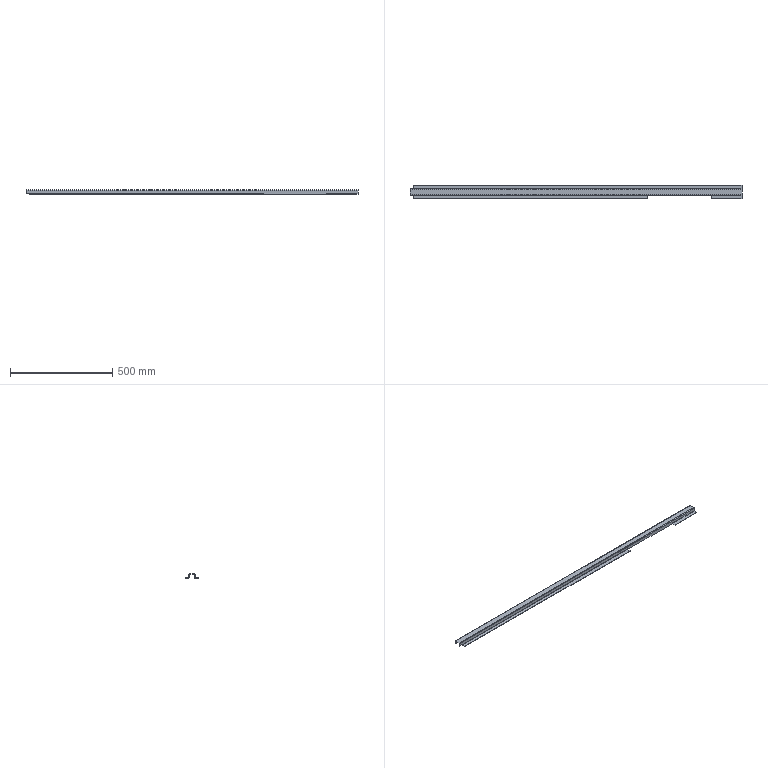Part | SolidWorks | features BaseBody 1 | 1 solid | 61 faces | box 1623 x 66 x 20 mm | volume 307877 mm3 | plane 51 | cylinder 10 | commonest cylinder face diameters 2 x5 6 x5